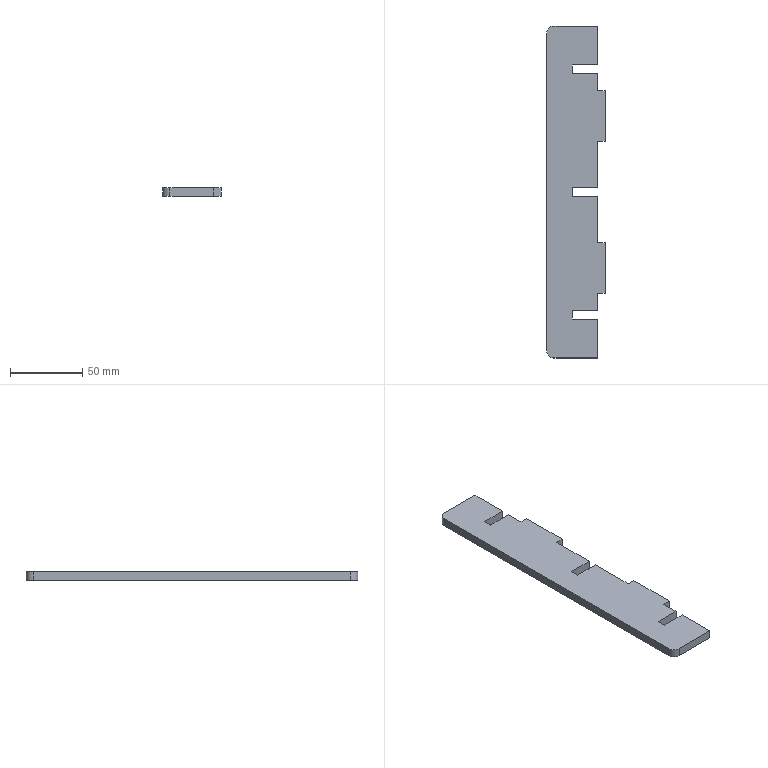Part | SolidWorks | features FlatPattern 1, SMBaseFlange 1, SheetMetal 1 | 1 solid | 28 faces | box 40.5 x 230 x 6 mm | volume 48656 mm3 | plane 26 | cylinder 2 | commonest cylinder face diameters 10 x2
STEP:
#1=CARTESIAN_POINT('',(-343.504,69.325,0.));
#2=VERTEX_POINT('',#1);
#3=CARTESIAN_POINT('',(-343.504,96.325,0.));
#4=VERTEX_POINT('',#3);
#5=CARTESIAN_POINT('',(-343.504,96.325,0.));
#6=DIRECTION('',(0.,1.,0.));
#7=VECTOR('',#6,1000.);
#8=LINE('',#5,#7);
#9=EDGE_CURVE('',#2,#4,#8,.T.);
#10=ORIENTED_EDGE('',*,*,#9,.F.);
#11=CARTESIAN_POINT('',(-343.504,69.325,-6.));
#12=VERTEX_POINT('',#11);
#13=CARTESIAN_POINT('',(-343.504,69.325,-6.));
#14=DIRECTION('',(0.,0.,1.));
#15=VECTOR('',#14,1000.);
#16=LINE('',#13,#15);
#17=EDGE_CURVE('',#12,#2,#16,.T.);
#18=ORIENTED_EDGE('',*,*,#17,.F.);
#19=CARTESIAN_POINT('',(-343.504,96.325,-6.));
#20=VERTEX_POINT('',#19);
#21=CARTESIAN_POINT('',(-343.504,96.325,-6.));
#22=DIRECTION('',(0.,1.,0.));
#23=VECTOR('',#22,1000.);
#24=LINE('',#21,#23);
#25=EDGE_CURVE('',#12,#20,#24,.T.);
#26=ORIENTED_EDGE('',*,*,#25,.T.);
#27=CARTESIAN_POINT('',(-343.504,96.325,-6.));
#28=DIRECTION('',(0.,0.,1.));
#29=VECTOR('',#28,1000.);
#30=LINE('',#27,#29);
#31=EDGE_CURVE('',#20,#4,#30,.T.);
#32=ORIENTED_EDGE('',*,*,#31,.T.);
#33=EDGE_LOOP('',(#10,#18,#26,#32));
#34=FACE_OUTER_BOUND('',#33,.T.);
#35=CARTESIAN_POINT('',(-343.504,96.325,-6.));
#36=DIRECTION('',(1.,0.,0.));
#37=DIRECTION('',(0.,1.,0.));
#38=AXIS2_PLACEMENT_3D('',#35,#36,#37);
#39=PLANE('',#38);
#40=ADVANCED_FACE('',(#34),#39,.T.);
#41=CARTESIAN_POINT('',(-361.004,69.325,0.));
#42=VERTEX_POINT('',#41);
#43=CARTESIAN_POINT('',(-343.504,69.325,0.));
#44=DIRECTION('',(1.,0.,0.));
#45=VECTOR('',#44,1000.);
#46=LINE('',#43,#45);
#47=EDGE_CURVE('',#42,#2,#46,.T.);
#48=ORIENTED_EDGE('',*,*,#47,.F.);
#49=CARTESIAN_POINT('',(-361.004,69.325,-6.));
#50=VERTEX_POINT('',#49);
#51=CARTESIAN_POINT('',(-361.004,69.325,-6.));
#52=DIRECTION('',(0.,0.,1.));
#53=VECTOR('',#52,1000.);
#54=LINE('',#51,#53);
#55=EDGE_CURVE('',#50,#42,#54,.T.);
#56=ORIENTED_EDGE('',*,*,#55,.F.);
#57=CARTESIAN_POINT('',(-343.504,69.325,-6.));
#58=DIRECTION('',(1.,0.,0.));
#59=VECTOR('',#58,1000.);
#60=LINE('',#57,#59);
#61=EDGE_CURVE('',#50,#12,#60,.T.);
#62=ORIENTED_EDGE('',*,*,#61,.T.);
#63=ORIENTED_EDGE('',*,*,#17,.T.);
#64=EDGE_LOOP('',(#48,#56,#62,#63));
#65=FACE_OUTER_BOUND('',#64,.T.);
#66=CARTESIAN_POINT('',(-343.504,69.325,-6.));
#67=DIRECTION('',(0.,-1.,0.));
#68=DIRECTION('',(0.,0.,-1.));
#69=AXIS2_PLACEMENT_3D('',#66,#67,#68);
#70=PLANE('',#69);
#71=ADVANCED_FACE('',(#65),#70,.T.);
#72=CARTESIAN_POINT('',(-361.004,63.325,0.));
#73=VERTEX_POINT('',#72);
#74=CARTESIAN_POINT('',(-361.004,69.325,0.));
#75=DIRECTION('',(0.,1.,0.));
#76=VECTOR('',#75,1000.);
#77=LINE('',#74,#76);
#78=EDGE_CURVE('',#73,#42,#77,.T.);
#79=ORIENTED_EDGE('',*,*,#78,.F.);
#80=CARTESIAN_POINT('',(-361.004,63.325,-6.));
#81=VERTEX_POINT('',#80);
#82=CARTESIAN_POINT('',(-361.004,63.325,-6.));
#83=DIRECTION('',(0.,0.,1.));
#84=VECTOR('',#83,1000.);
#85=LINE('',#82,#84);
#86=EDGE_CURVE('',#81,#73,#85,.T.);
#87=ORIENTED_EDGE('',*,*,#86,.F.);
#88=CARTESIAN_POINT('',(-361.004,69.325,-6.));
#89=DIRECTION('',(0.,1.,0.));
#90=VECTOR('',#89,1000.);
#91=LINE('',#88,#90);
#92=EDGE_CURVE('',#81,#50,#91,.T.);
#93=ORIENTED_EDGE('',*,*,#92,.T.);
#94=ORIENTED_EDGE('',*,*,#55,.T.);
#95=EDGE_LOOP('',(#79,#87,#93,#94));
#96=FACE_OUTER_BOUND('',#95,.T.);
#97=CARTESIAN_POINT('',(-361.004,69.325,-6.));
#98=DIRECTION('',(1.,0.,0.));
#99=DIRECTION('',(0.,0.,-1.));
#100=AXIS2_PLACEMENT_3D('',#97,#98,#99);
#101=PLANE('',#100);
#102=ADVANCED_FACE('',(#96),#101,.T.);
#103=CARTESIAN_POINT('',(-343.504,63.325,0.));
#104=VERTEX_POINT('',#103);
#105=CARTESIAN_POINT('',(-361.004,63.325,0.));
#106=DIRECTION('',(-1.,0.,0.));
#107=VECTOR('',#106,1000.);
#108=LINE('',#105,#107);
#109=EDGE_CURVE('',#104,#73,#108,.T.);
#110=ORIENTED_EDGE('',*,*,#109,.F.);
#111=CARTESIAN_POINT('',(-343.504,63.325,-6.));
#112=VERTEX_POINT('',#111);
#113=CARTESIAN_POINT('',(-343.504,63.325,-6.));
#114=DIRECTION('',(0.,0.,1.));
#115=VECTOR('',#114,1000.);
#116=LINE('',#113,#115);
#117=EDGE_CURVE('',#112,#104,#116,.T.);
#118=ORIENTED_EDGE('',*,*,#117,.F.);
#119=CARTESIAN_POINT('',(-361.004,63.325,-6.));
#120=DIRECTION('',(-1.,0.,0.));
#121=VECTOR('',#120,1000.);
#122=LINE('',#119,#121);
#123=EDGE_CURVE('',#112,#81,#122,.T.);
#124=ORIENTED_EDGE('',*,*,#123,.T.);
#125=ORIENTED_EDGE('',*,*,#86,.T.);
#126=EDGE_LOOP('',(#110,#118,#124,#125));
#127=FACE_OUTER_BOUND('',#126,.T.);
#128=CARTESIAN_POINT('',(-361.004,63.325,-6.));
#129=DIRECTION('',(0.,1.,0.));
#130=DIRECTION('',(0.,0.,1.));
#131=AXIS2_PLACEMENT_3D('',#128,#129,#130);
#132=PLANE('',#131);
#133=ADVANCED_FACE('',(#127),#132,.T.);
#134=CARTESIAN_POINT('',(-343.504,51.325,0.));
#135=VERTEX_POINT('',#134);
#136=CARTESIAN_POINT('',(-343.504,63.325,0.));
#137=DIRECTION('',(0.,1.,0.));
#138=VECTOR('',#137,1000.);
#139=LINE('',#136,#138);
#140=EDGE_CURVE('',#135,#104,#139,.T.);
#141=ORIENTED_EDGE('',*,*,#140,.F.);
#142=CARTESIAN_POINT('',(-343.504,51.325,-6.));
#143=VERTEX_POINT('',#142);
#144=CARTESIAN_POINT('',(-343.504,51.325,-6.));
#145=DIRECTION('',(0.,0.,1.));
#146=VECTOR('',#145,1000.);
#147=LINE('',#144,#146);
#148=EDGE_CURVE('',#143,#135,#147,.T.);
#149=ORIENTED_EDGE('',*,*,#148,.F.);
#150=CARTESIAN_POINT('',(-343.504,63.325,-6.));
#151=DIRECTION('',(0.,1.,0.));
#152=VECTOR('',#151,1000.);
#153=LINE('',#150,#152);
#154=EDGE_CURVE('',#143,#112,#153,.T.);
#155=ORIENTED_EDGE('',*,*,#154,.T.);
#156=ORIENTED_EDGE('',*,*,#117,.T.);
#157=EDGE_LOOP('',(#141,#149,#155,#156));
#158=FACE_OUTER_BOUND('',#157,.T.);
#159=CARTESIAN_POINT('',(-343.504,63.325,-6.));
#160=DIRECTION('',(1.,0.,0.));
#161=DIRECTION('',(0.,1.,0.));
#162=AXIS2_PLACEMENT_3D('',#159,#160,#161);
#163=PLANE('',#162);
#164=ADVANCED_FACE('',(#158),#163,.T.);
#165=CARTESIAN_POINT('',(-338.004,51.325,0.));
#166=VERTEX_POINT('',#165);
#167=CARTESIAN_POINT('',(-343.504,51.325,0.));
#168=DIRECTION('',(-1.,0.,0.));
#169=VECTOR('',#168,1000.);
#170=LINE('',#167,#169);
#171=EDGE_CURVE('',#166,#135,#170,.T.);
#172=ORIENTED_EDGE('',*,*,#171,.F.);
#173=CARTESIAN_POINT('',(-338.004,51.325,-6.));
#174=VERTEX_POINT('',#173);
#175=CARTESIAN_POINT('',(-338.004,51.325,-6.));
#176=DIRECTION('',(0.,0.,1.));
#177=VECTOR('',#176,1000.);
#178=LINE('',#175,#177);
#179=EDGE_CURVE('',#174,#166,#178,.T.);
#180=ORIENTED_EDGE('',*,*,#179,.F.);
#181=CARTESIAN_POINT('',(-343.504,51.325,-6.));
#182=DIRECTION('',(-1.,0.,0.));
#183=VECTOR('',#182,1000.);
#184=LINE('',#181,#183);
#185=EDGE_CURVE('',#174,#143,#184,.T.);
#186=ORIENTED_EDGE('',*,*,#185,.T.);
#187=ORIENTED_EDGE('',*,*,#148,.T.);
#188=EDGE_LOOP('',(#172,#180,#186,#187));
#189=FACE_OUTER_BOUND('',#188,.T.);
#190=CARTESIAN_POINT('',(-343.504,51.325,-6.));
#191=DIRECTION('',(0.,1.,0.));
#192=DIRECTION('',(-1.,0.,0.));
#193=AXIS2_PLACEMENT_3D('',#190,#191,#192);
#194=PLANE('',#193);
#195=ADVANCED_FACE('',(#189),#194,.T.);
#196=CARTESIAN_POINT('',(-338.004,16.325,0.));
#197=VERTEX_POINT('',#196);
#198=CARTESIAN_POINT('',(-338.004,51.325,0.));
#199=DIRECTION('',(0.,1.,0.));
#200=VECTOR('',#199,1000.);
#201=LINE('',#198,#200);
#202=EDGE_CURVE('',#197,#166,#201,.T.);
#203=ORIENTED_EDGE('',*,*,#202,.F.);
#204=CARTESIAN_POINT('',(-338.004,16.325,-6.));
#205=VERTEX_POINT('',#204);
#206=CARTESIAN_POINT('',(-338.004,16.325,-6.));
#207=DIRECTION('',(0.,0.,1.));
#208=VECTOR('',#207,1000.);
#209=LINE('',#206,#208);
#210=EDGE_CURVE('',#205,#197,#209,.T.);
#211=ORIENTED_EDGE('',*,*,#210,.F.);
#212=CARTESIAN_POINT('',(-338.004,51.325,-6.));
#213=DIRECTION('',(0.,1.,0.));
#214=VECTOR('',#213,1000.);
#215=LINE('',#212,#214);
#216=EDGE_CURVE('',#205,#174,#215,.T.);
#217=ORIENTED_EDGE('',*,*,#216,.T.);
#218=ORIENTED_EDGE('',*,*,#179,.T.);
#219=EDGE_LOOP('',(#203,#211,#217,#218));
#220=FACE_OUTER_BOUND('',#219,.T.);
#221=CARTESIAN_POINT('',(-338.004,51.325,-6.));
#222=DIRECTION('',(1.,0.,0.));
#223=DIRECTION('',(0.,0.,-1.));
#224=AXIS2_PLACEMENT_3D('',#221,#222,#223);
#225=PLANE('',#224);
#226=ADVANCED_FACE('',(#220),#225,.T.);
#227=CARTESIAN_POINT('',(-343.504,16.325,0.));
#228=VERTEX_POINT('',#227);
#229=CARTESIAN_POINT('',(-338.004,16.325,0.));
#230=DIRECTION('',(1.,0.,0.));
#231=VECTOR('',#230,1000.);
#232=LINE('',#229,#231);
#233=EDGE_CURVE('',#228,#197,#232,.T.);
#234=ORIENTED_EDGE('',*,*,#233,.F.);
#235=CARTESIAN_POINT('',(-343.504,16.325,-6.));
#236=VERTEX_POINT('',#235);
#237=CARTESIAN_POINT('',(-343.504,16.325,-6.));
#238=DIRECTION('',(0.,0.,1.));
#239=VECTOR('',#238,1000.);
#240=LINE('',#237,#239);
#241=EDGE_CURVE('',#236,#228,#240,.T.);
#242=ORIENTED_EDGE('',*,*,#241,.F.);
#243=CARTESIAN_POINT('',(-338.004,16.325,-6.));
#244=DIRECTION('',(1.,0.,0.));
#245=VECTOR('',#244,1000.);
#246=LINE('',#243,#245);
#247=EDGE_CURVE('',#236,#205,#246,.T.);
#248=ORIENTED_EDGE('',*,*,#247,.T.);
#249=ORIENTED_EDGE('',*,*,#210,.T.);
#250=EDGE_LOOP('',(#234,#242,#248,#249));
#251=FACE_OUTER_BOUND('',#250,.T.);
#252=CARTESIAN_POINT('',(-338.004,16.325,-6.));
#253=DIRECTION('',(0.,-1.,0.));
#254=DIRECTION('',(0.,0.,-1.));
#255=AXIS2_PLACEMENT_3D('',#252,#253,#254);
#256=PLANE('',#255);
#257=ADVANCED_FACE('',(#251),#256,.T.);
#258=CARTESIAN_POINT('',(-343.504,-15.675,0.));
#259=VERTEX_POINT('',#258);
#260=CARTESIAN_POINT('',(-343.504,16.325,0.));
#261=DIRECTION('',(0.,1.,0.));
#262=VECTOR('',#261,1000.);
#263=LINE('',#260,#262);
#264=EDGE_CURVE('',#259,#228,#263,.T.);
#265=ORIENTED_EDGE('',*,*,#264,.F.);
#266=CARTESIAN_POINT('',(-343.504,-15.675,-6.));
#267=VERTEX_POINT('',#266);
#268=CARTESIAN_POINT('',(-343.504,-15.675,-6.));
#269=DIRECTION('',(0.,0.,1.));
#270=VECTOR('',#269,1000.);
#271=LINE('',#268,#270);
#272=EDGE_CURVE('',#267,#259,#271,.T.);
#273=ORIENTED_EDGE('',*,*,#272,.F.);
#274=CARTESIAN_POINT('',(-343.504,16.325,-6.));
#275=DIRECTION('',(0.,1.,0.));
#276=VECTOR('',#275,1000.);
#277=LINE('',#274,#276);
#278=EDGE_CURVE('',#267,#236,#277,.T.);
#279=ORIENTED_EDGE('',*,*,#278,.T.);
#280=ORIENTED_EDGE('',*,*,#241,.T.);
#281=EDGE_LOOP('',(#265,#273,#279,#280));
#282=FACE_OUTER_BOUND('',#281,.T.);
#283=CARTESIAN_POINT('',(-343.504,16.325,-6.));
#284=DIRECTION('',(1.,0.,0.));
#285=DIRECTION('',(0.,1.,0.));
#286=AXIS2_PLACEMENT_3D('',#283,#284,#285);
#287=PLANE('',#286);
#288=ADVANCED_FACE('',(#282),#287,.T.);
#289=CARTESIAN_POINT('',(-361.004,-15.675,0.));
#290=VERTEX_POINT('',#289);
#291=CARTESIAN_POINT('',(-343.504,-15.675,0.));
#292=DIRECTION('',(1.,0.,0.));
#293=VECTOR('',#292,1000.);
#294=LINE('',#291,#293);
#295=EDGE_CURVE('',#290,#259,#294,.T.);
#296=ORIENTED_EDGE('',*,*,#295,.F.);
#297=CARTESIAN_POINT('',(-361.004,-15.675,-6.));
#298=VERTEX_POINT('',#297);
#299=CARTESIAN_POINT('',(-361.004,-15.675,-6.));
#300=DIRECTION('',(0.,0.,1.));
#301=VECTOR('',#300,1000.);
#302=LINE('',#299,#301);
#303=EDGE_CURVE('',#298,#290,#302,.T.);
#304=ORIENTED_EDGE('',*,*,#303,.F.);
#305=CARTESIAN_POINT('',(-343.504,-15.675,-6.));
#306=DIRECTION('',(1.,0.,0.));
#307=VECTOR('',#306,1000.);
#308=LINE('',#305,#307);
#309=EDGE_CURVE('',#298,#267,#308,.T.);
#310=ORIENTED_EDGE('',*,*,#309,.T.);
#311=ORIENTED_EDGE('',*,*,#272,.T.);
#312=EDGE_LOOP('',(#296,#304,#310,#311));
#313=FACE_OUTER_BOUND('',#312,.T.);
#314=CARTESIAN_POINT('',(-343.504,-15.675,-6.));
#315=DIRECTION('',(0.,-1.,0.));
#316=DIRECTION('',(0.,0.,-1.));
#317=AXIS2_PLACEMENT_3D('',#314,#315,#316);
#318=PLANE('',#317);
#319=ADVANCED_FACE('',(#313),#318,.T.);
#320=CARTESIAN_POINT('',(-361.004,-21.675,0.));
#321=VERTEX_POINT('',#320);
#322=CARTESIAN_POINT('',(-361.004,-15.675,0.));
#323=DIRECTION('',(0.,1.,0.));
#324=VECTOR('',#323,1000.);
#325=LINE('',#322,#324);
#326=EDGE_CURVE('',#321,#290,#325,.T.);
#327=ORIENTED_EDGE('',*,*,#326,.F.);
#328=CARTESIAN_POINT('',(-361.004,-21.675,-6.));
#329=VERTEX_POINT('',#328);
#330=CARTESIAN_POINT('',(-361.004,-21.675,-6.));
#331=DIRECTION('',(0.,0.,1.));
#332=VECTOR('',#331,1000.);
#333=LINE('',#330,#332);
#334=EDGE_CURVE('',#329,#321,#333,.T.);
#335=ORIENTED_EDGE('',*,*,#334,.F.);
#336=CARTESIAN_POINT('',(-361.004,-15.675,-6.));
#337=DIRECTION('',(0.,1.,0.));
#338=VECTOR('',#337,1000.);
#339=LINE('',#336,#338);
#340=EDGE_CURVE('',#329,#298,#339,.T.);
#341=ORIENTED_EDGE('',*,*,#340,.T.);
#342=ORIENTED_EDGE('',*,*,#303,.T.);
#343=EDGE_LOOP('',(#327,#335,#341,#342));
#344=FACE_OUTER_BOUND('',#343,.T.);
#345=CARTESIAN_POINT('',(-361.004,-15.675,-6.));
#346=DIRECTION('',(1.,0.,0.));
#347=DIRECTION('',(0.,0.,-1.));
#348=AXIS2_PLACEMENT_3D('',#345,#346,#347);
#349=PLANE('',#348);
#350=ADVANCED_FACE('',(#344),#349,.T.);
#351=CARTESIAN_POINT('',(-343.504,-21.675,0.));
#352=VERTEX_POINT('',#351);
#353=CARTESIAN_POINT('',(-361.004,-21.675,0.));
#354=DIRECTION('',(-1.,0.,0.));
#355=VECTOR('',#354,1000.);
#356=LINE('',#353,#355);
#357=EDGE_CURVE('',#352,#321,#356,.T.);
#358=ORIENTED_EDGE('',*,*,#357,.F.);
#359=CARTESIAN_POINT('',(-343.504,-21.675,-6.));
#360=VERTEX_POINT('',#359);
#361=CARTESIAN_POINT('',(-343.504,-21.675,-6.));
#362=DIRECTION('',(0.,0.,1.));
#363=VECTOR('',#362,1000.);
#364=LINE('',#361,#363);
#365=EDGE_CURVE('',#360,#352,#364,.T.);
#366=ORIENTED_EDGE('',*,*,#365,.F.);
#367=CARTESIAN_POINT('',(-361.004,-21.675,-6.));
#368=DIRECTION('',(-1.,0.,0.));
#369=VECTOR('',#368,1000.);
#370=LINE('',#367,#369);
#371=EDGE_CURVE('',#360,#329,#370,.T.);
#372=ORIENTED_EDGE('',*,*,#371,.T.);
#373=ORIENTED_EDGE('',*,*,#334,.T.);
#374=EDGE_LOOP('',(#358,#366,#372,#373));
#375=FACE_OUTER_BOUND('',#374,.T.);
#376=CARTESIAN_POINT('',(-361.004,-21.675,-6.));
#377=DIRECTION('',(0.,1.,0.));
#378=DIRECTION('',(0.,0.,1.));
#379=AXIS2_PLACEMENT_3D('',#376,#377,#378);
#380=PLANE('',#379);
#381=ADVANCED_FACE('',(#375),#380,.T.);
#382=CARTESIAN_POINT('',(-343.504,-53.675,0.));
#383=VERTEX_POINT('',#382);
#384=CARTESIAN_POINT('',(-343.504,-21.675,0.));
#385=DIRECTION('',(0.,1.,0.));
#386=VECTOR('',#385,1000.);
#387=LINE('',#384,#386);
#388=EDGE_CURVE('',#383,#352,#387,.T.);
#389=ORIENTED_EDGE('',*,*,#388,.F.);
#390=CARTESIAN_POINT('',(-343.504,-53.675,-6.));
#391=VERTEX_POINT('',#390);
#392=CARTESIAN_POINT('',(-343.504,-53.675,-6.));
#393=DIRECTION('',(0.,0.,1.));
#394=VECTOR('',#393,1000.);
#395=LINE('',#392,#394);
#396=EDGE_CURVE('',#391,#383,#395,.T.);
#397=ORIENTED_EDGE('',*,*,#396,.F.);
#398=CARTESIAN_POINT('',(-343.504,-21.675,-6.));
#399=DIRECTION('',(0.,1.,0.));
#400=VECTOR('',#399,1000.);
#401=LINE('',#398,#400);
#402=EDGE_CURVE('',#391,#360,#401,.T.);
#403=ORIENTED_EDGE('',*,*,#402,.T.);
#404=ORIENTED_EDGE('',*,*,#365,.T.);
#405=EDGE_LOOP('',(#389,#397,#403,#404));
#406=FACE_OUTER_BOUND('',#405,.T.);
#407=CARTESIAN_POINT('',(-343.504,-21.675,-6.));
#408=DIRECTION('',(1.,0.,0.));
#409=DIRECTION('',(0.,1.,0.));
#410=AXIS2_PLACEMENT_3D('',#407,#408,#409);
#411=PLANE('',#410);
#412=ADVANCED_FACE('',(#406),#411,.T.);
#413=CARTESIAN_POINT('',(-338.004,-53.675,0.));
#414=VERTEX_POINT('',#413);
#415=CARTESIAN_POINT('',(-343.504,-53.675,0.));
#416=DIRECTION('',(-1.,0.,0.));
#417=VECTOR('',#416,1000.);
#418=LINE('',#415,#417);
#419=EDGE_CURVE('',#414,#383,#418,.T.);
#420=ORIENTED_EDGE('',*,*,#419,.F.);
#421=CARTESIAN_POINT('',(-338.004,-53.675,-6.));
#422=VERTEX_POINT('',#421);
#423=CARTESIAN_POINT('',(-338.004,-53.675,-6.));
#424=DIRECTION('',(0.,0.,1.));
#425=VECTOR('',#424,1000.);
#426=LINE('',#423,#425);
#427=EDGE_CURVE('',#422,#414,#426,.T.);
#428=ORIENTED_EDGE('',*,*,#427,.F.);
#429=CARTESIAN_POINT('',(-343.504,-53.675,-6.));
#430=DIRECTION('',(-1.,0.,0.));
#431=VECTOR('',#430,1000.);
#432=LINE('',#429,#431);
#433=EDGE_CURVE('',#422,#391,#432,.T.);
#434=ORIENTED_EDGE('',*,*,#433,.T.);
#435=ORIENTED_EDGE('',*,*,#396,.T.);
#436=EDGE_LOOP('',(#420,#428,#434,#435));
#437=FACE_OUTER_BOUND('',#436,.T.);
#438=CARTESIAN_POINT('',(-343.504,-53.675,-6.));
#439=DIRECTION('',(0.,1.,0.));
#440=DIRECTION('',(0.,0.,1.));
#441=AXIS2_PLACEMENT_3D('',#438,#439,#440);
#442=PLANE('',#441);
#443=ADVANCED_FACE('',(#437),#442,.T.);
#444=CARTESIAN_POINT('',(-338.004,-88.675,0.));
#445=VERTEX_POINT('',#444);
#446=CARTESIAN_POINT('',(-338.004,-53.675,0.));
#447=DIRECTION('',(0.,1.,0.));
#448=VECTOR('',#447,1000.);
#449=LINE('',#446,#448);
#450=EDGE_CURVE('',#445,#414,#449,.T.);
#451=ORIENTED_EDGE('',*,*,#450,.F.);
#452=CARTESIAN_POINT('',(-338.004,-88.675,-6.));
#453=VERTEX_POINT('',#452);
#454=CARTESIAN_POINT('',(-338.004,-88.675,-6.));
#455=DIRECTION('',(0.,0.,1.));
#456=VECTOR('',#455,1000.);
#457=LINE('',#454,#456);
#458=EDGE_CURVE('',#453,#445,#457,.T.);
#459=ORIENTED_EDGE('',*,*,#458,.F.);
#460=CARTESIAN_POINT('',(-338.004,-53.675,-6.));
#461=DIRECTION('',(0.,1.,0.));
#462=VECTOR('',#461,1000.);
#463=LINE('',#460,#462);
#464=EDGE_CURVE('',#453,#422,#463,.T.);
#465=ORIENTED_EDGE('',*,*,#464,.T.);
#466=ORIENTED_EDGE('',*,*,#427,.T.);
#467=EDGE_LOOP('',(#451,#459,#465,#466));
#468=FACE_OUTER_BOUND('',#467,.T.);
#469=CARTESIAN_POINT('',(-338.004,-53.675,-6.));
#470=DIRECTION('',(1.,0.,0.));
#471=DIRECTION('',(0.,0.,-1.));
#472=AXIS2_PLACEMENT_3D('',#469,#470,#471);
#473=PLANE('',#472);
#474=ADVANCED_FACE('',(#468),#473,.T.);
#475=CARTESIAN_POINT('',(-343.504,-88.675,0.));
#476=VERTEX_POINT('',#475);
#477=CARTESIAN_POINT('',(-338.004,-88.675,0.));
#478=DIRECTION('',(1.,0.,0.));
#479=VECTOR('',#478,1000.);
#480=LINE('',#477,#479);
#481=EDGE_CURVE('',#476,#445,#480,.T.);
#482=ORIENTED_EDGE('',*,*,#481,.F.);
#483=CARTESIAN_POINT('',(-343.504,-88.675,-6.));
#484=VERTEX_POINT('',#483);
#485=CARTESIAN_POINT('',(-343.504,-88.675,-6.));
#486=DIRECTION('',(0.,0.,1.));
#487=VECTOR('',#486,1000.);
#488=LINE('',#485,#487);
#489=EDGE_CURVE('',#484,#476,#488,.T.);
#490=ORIENTED_EDGE('',*,*,#489,.F.);
#491=CARTESIAN_POINT('',(-338.004,-88.675,-6.));
#492=DIRECTION('',(1.,0.,0.));
#493=VECTOR('',#492,1000.);
#494=LINE('',#491,#493);
#495=EDGE_CURVE('',#484,#453,#494,.T.);
#496=ORIENTED_EDGE('',*,*,#495,.T.);
#497=ORIENTED_EDGE('',*,*,#458,.T.);
#498=EDGE_LOOP('',(#482,#490,#496,#497));
#499=FACE_OUTER_BOUND('',#498,.T.);
#500=CARTESIAN_POINT('',(-338.004,-88.675,-6.));
#501=DIRECTION('',(0.,-1.,0.));
#502=DIRECTION('',(0.,0.,-1.));
#503=AXIS2_PLACEMENT_3D('',#500,#501,#502);
#504=PLANE('',#503);
#505=ADVANCED_FACE('',(#499),#504,.T.);
#506=CARTESIAN_POINT('',(-343.504,-100.675,0.));
#507=VERTEX_POINT('',#506);
#508=CARTESIAN_POINT('',(-343.504,-88.675,0.));
#509=DIRECTION('',(0.,1.,0.));
#510=VECTOR('',#509,1000.);
#511=LINE('',#508,#510);
#512=EDGE_CURVE('',#507,#476,#511,.T.);
#513=ORIENTED_EDGE('',*,*,#512,.F.);
#514=CARTESIAN_POINT('',(-343.504,-100.675,-6.));
#515=VERTEX_POINT('',#514);
#516=CARTESIAN_POINT('',(-343.504,-100.675,-6.));
#517=DIRECTION('',(0.,0.,1.));
#518=VECTOR('',#517,1000.);
#519=LINE('',#516,#518);
#520=EDGE_CURVE('',#515,#507,#519,.T.);
#521=ORIENTED_EDGE('',*,*,#520,.F.);
#522=CARTESIAN_POINT('',(-343.504,-88.675,-6.));
#523=DIRECTION('',(0.,1.,0.));
#524=VECTOR('',#523,1000.);
#525=LINE('',#522,#524);
#526=EDGE_CURVE('',#515,#484,#525,.T.);
#527=ORIENTED_EDGE('',*,*,#526,.T.);
#528=ORIENTED_EDGE('',*,*,#489,.T.);
#529=EDGE_LOOP('',(#513,#521,#527,#528));
#530=FACE_OUTER_BOUND('',#529,.T.);
#531=CARTESIAN_POINT('',(-343.504,-88.675,-6.));
#532=DIRECTION('',(1.,0.,0.));
#533=DIRECTION('',(0.,0.,-1.));
#534=AXIS2_PLACEMENT_3D('',#531,#532,#533);
#535=PLANE('',#534);
#536=ADVANCED_FACE('',(#530),#535,.T.);
#537=CARTESIAN_POINT('',(-361.004,-100.675,0.));
#538=VERTEX_POINT('',#537);
#539=CARTESIAN_POINT('',(-343.504,-100.675,0.));
#540=DIRECTION('',(1.,0.,0.));
#541=VECTOR('',#540,1000.);
#542=LINE('',#539,#541);
#543=EDGE_CURVE('',#538,#507,#542,.T.);
#544=ORIENTED_EDGE('',*,*,#543,.F.);
#545=CARTESIAN_POINT('',(-361.004,-100.675,-6.));
#546=VERTEX_POINT('',#545);
#547=CARTESIAN_POINT('',(-361.004,-100.675,-6.));
#548=DIRECTION('',(0.,0.,1.));
#549=VECTOR('',#548,1000.);
#550=LINE('',#547,#549);
#551=EDGE_CURVE('',#546,#538,#550,.T.);
#552=ORIENTED_EDGE('',*,*,#551,.F.);
#553=CARTESIAN_POINT('',(-343.504,-100.675,-6.));
#554=DIRECTION('',(1.,0.,0.));
#555=VECTOR('',#554,1000.);
#556=LINE('',#553,#555);
#557=EDGE_CURVE('',#546,#515,#556,.T.);
#558=ORIENTED_EDGE('',*,*,#557,.T.);
#559=ORIENTED_EDGE('',*,*,#520,.T.);
#560=EDGE_LOOP('',(#544,#552,#558,#559));
#561=FACE_OUTER_BOUND('',#560,.T.);
#562=CARTESIAN_POINT('',(-343.504,-100.675,-6.));
#563=DIRECTION('',(0.,-1.,0.));
#564=DIRECTION('',(0.,0.,-1.));
#565=AXIS2_PLACEMENT_3D('',#562,#563,#564);
#566=PLANE('',#565);
#567=ADVANCED_FACE('',(#561),#566,.T.);
#568=CARTESIAN_POINT('',(-361.004,-106.675,0.));
#569=VERTEX_POINT('',#568);
#570=CARTESIAN_POINT('',(-361.004,-100.675,0.));
#571=DIRECTION('',(0.,1.,0.));
#572=VECTOR('',#571,1000.);
#573=LINE('',#570,#572);
#574=EDGE_CURVE('',#569,#538,#573,.T.);
#575=ORIENTED_EDGE('',*,*,#574,.F.);
#576=CARTESIAN_POINT('',(-361.004,-106.675,-6.));
#577=VERTEX_POINT('',#576);
#578=CARTESIAN_POINT('',(-361.004,-106.675,-6.));
#579=DIRECTION('',(0.,0.,1.));
#580=VECTOR('',#579,1000.);
#581=LINE('',#578,#580);
#582=EDGE_CURVE('',#577,#569,#581,.T.);
#583=ORIENTED_EDGE('',*,*,#582,.F.);
#584=CARTESIAN_POINT('',(-361.004,-100.675,-6.));
#585=DIRECTION('',(0.,1.,0.));
#586=VECTOR('',#585,1000.);
#587=LINE('',#584,#586);
#588=EDGE_CURVE('',#577,#546,#587,.T.);
#589=ORIENTED_EDGE('',*,*,#588,.T.);
#590=ORIENTED_EDGE('',*,*,#551,.T.);
#591=EDGE_LOOP('',(#575,#583,#589,#590));
#592=FACE_OUTER_BOUND('',#591,.T.);
#593=CARTESIAN_POINT('',(-361.004,-100.675,-6.));
#594=DIRECTION('',(1.,0.,0.));
#595=DIRECTION('',(0.,0.,-1.));
#596=AXIS2_PLACEMENT_3D('',#593,#594,#595);
#597=PLANE('',#596);
#598=ADVANCED_FACE('',(#592),#597,.T.);
#599=CARTESIAN_POINT('',(-343.504,-106.675,0.));
#600=VERTEX_POINT('',#599);
#601=CARTESIAN_POINT('',(-361.004,-106.675,0.));
#602=DIRECTION('',(-1.,0.,0.));
#603=VECTOR('',#602,1000.);
#604=LINE('',#601,#603);
#605=EDGE_CURVE('',#600,#569,#604,.T.);
#606=ORIENTED_EDGE('',*,*,#605,.F.);
#607=CARTESIAN_POINT('',(-343.504,-106.675,-6.));
#608=VERTEX_POINT('',#607);
#609=CARTESIAN_POINT('',(-343.504,-106.675,-6.));
#610=DIRECTION('',(0.,0.,1.));
#611=VECTOR('',#610,1000.);
#612=LINE('',#609,#611);
#613=EDGE_CURVE('',#608,#600,#612,.T.);
#614=ORIENTED_EDGE('',*,*,#613,.F.);
#615=CARTESIAN_POINT('',(-361.004,-106.675,-6.));
#616=DIRECTION('',(-1.,0.,0.));
#617=VECTOR('',#616,1000.);
#618=LINE('',#615,#617);
#619=EDGE_CURVE('',#608,#577,#618,.T.);
#620=ORIENTED_EDGE('',*,*,#619,.T.);
#621=ORIENTED_EDGE('',*,*,#582,.T.);
#622=EDGE_LOOP('',(#606,#614,#620,#621));
#623=FACE_OUTER_BOUND('',#622,.T.);
#624=CARTESIAN_POINT('',(-361.004,-106.675,-6.));
#625=DIRECTION('',(0.,1.,0.));
#626=DIRECTION('',(0.,0.,1.));
#627=AXIS2_PLACEMENT_3D('',#624,#625,#626);
#628=PLANE('',#627);
#629=ADVANCED_FACE('',(#623),#628,.T.);
#630=CARTESIAN_POINT('',(-343.504,-133.675,0.));
#631=VERTEX_POINT('',#630);
#632=CARTESIAN_POINT('',(-343.504,-106.675,0.));
#633=DIRECTION('',(0.,1.,0.));
#634=VECTOR('',#633,1000.);
#635=LINE('',#632,#634);
#636=EDGE_CURVE('',#631,#600,#635,.T.);
#637=ORIENTED_EDGE('',*,*,#636,.F.);
#638=CARTESIAN_POINT('',(-343.504,-133.675,-6.));
#639=VERTEX_POINT('',#638);
#640=CARTESIAN_POINT('',(-343.504,-133.675,-6.));
#641=DIRECTION('',(0.,0.,1.));
#642=VECTOR('',#641,1000.);
#643=LINE('',#640,#642);
#644=EDGE_CURVE('',#639,#631,#643,.T.);
#645=ORIENTED_EDGE('',*,*,#644,.F.);
#646=CARTESIAN_POINT('',(-343.504,-106.675,-6.));
#647=DIRECTION('',(0.,1.,0.));
#648=VECTOR('',#647,1000.);
#649=LINE('',#646,#648);
#650=EDGE_CURVE('',#639,#608,#649,.T.);
#651=ORIENTED_EDGE('',*,*,#650,.T.);
#652=ORIENTED_EDGE('',*,*,#613,.T.);
#653=EDGE_LOOP('',(#637,#645,#651,#652));
#654=FACE_OUTER_BOUND('',#653,.T.);
#655=CARTESIAN_POINT('',(-343.504,-106.675,-6.));
#656=DIRECTION('',(1.,0.,0.));
#657=DIRECTION('',(0.,0.,-1.));
#658=AXIS2_PLACEMENT_3D('',#655,#656,#657);
#659=PLANE('',#658);
#660=ADVANCED_FACE('',(#654),#659,.T.);
#661=CARTESIAN_POINT('',(-373.504,-133.675,0.));
#662=VERTEX_POINT('',#661);
#663=CARTESIAN_POINT('',(-343.504,-133.675,0.));
#664=DIRECTION('',(1.,0.,0.));
#665=VECTOR('',#664,1000.);
#666=LINE('',#663,#665);
#667=EDGE_CURVE('',#662,#631,#666,.T.);
#668=ORIENTED_EDGE('',*,*,#667,.F.);
#669=CARTESIAN_POINT('',(-373.504,-133.675,-6.));
#670=VERTEX_POINT('',#669);
#671=CARTESIAN_POINT('',(-373.504,-133.675,-6.));
#672=DIRECTION('',(0.,0.,1.));
#673=VECTOR('',#672,1000.);
#674=LINE('',#671,#673);
#675=EDGE_CURVE('',#670,#662,#674,.T.);
#676=ORIENTED_EDGE('',*,*,#675,.F.);
#677=CARTESIAN_POINT('',(-343.504,-133.675,-6.));
#678=DIRECTION('',(1.,0.,0.));
#679=VECTOR('',#678,1000.);
#680=LINE('',#677,#679);
#681=EDGE_CURVE('',#670,#639,#680,.T.);
#682=ORIENTED_EDGE('',*,*,#681,.T.);
#683=ORIENTED_EDGE('',*,*,#644,.T.);
#684=EDGE_LOOP('',(#668,#676,#682,#683));
#685=FACE_OUTER_BOUND('',#684,.T.);
#686=CARTESIAN_POINT('',(-343.504,-133.675,-6.));
#687=DIRECTION('',(0.,-1.,0.));
#688=DIRECTION('',(0.,0.,-1.));
#689=AXIS2_PLACEMENT_3D('',#686,#687,#688);
#690=PLANE('',#689);
#691=ADVANCED_FACE('',(#685),#690,.T.);
#692=CARTESIAN_POINT('',(-378.504,-128.675,0.));
#693=VERTEX_POINT('',#692);
#694=CARTESIAN_POINT('',(-373.504,-128.675,0.));
#695=DIRECTION('',(0.,0.,1.));
#696=DIRECTION('',(-1.,0.,0.));
#697=AXIS2_PLACEMENT_3D('',#694,#695,#696);
#698=CIRCLE('',#697,5.);
#699=EDGE_CURVE('',#693,#662,#698,.T.);
#700=ORIENTED_EDGE('',*,*,#699,.F.);
#701=CARTESIAN_POINT('',(-378.504,-128.675,-6.));
#702=VERTEX_POINT('',#701);
#703=CARTESIAN_POINT('',(-378.504,-128.675,-6.));
#704=DIRECTION('',(0.,0.,1.));
#705=VECTOR('',#704,1000.);
#706=LINE('',#703,#705);
#707=EDGE_CURVE('',#702,#693,#706,.T.);
#708=ORIENTED_EDGE('',*,*,#707,.F.);
#709=CARTESIAN_POINT('',(-373.504,-128.675,-6.));
#710=DIRECTION('',(0.,0.,1.));
#711=DIRECTION('',(-1.,0.,0.));
#712=AXIS2_PLACEMENT_3D('',#709,#710,#711);
#713=CIRCLE('',#712,5.);
#714=EDGE_CURVE('',#702,#670,#713,.T.);
#715=ORIENTED_EDGE('',*,*,#714,.T.);
#716=ORIENTED_EDGE('',*,*,#675,.T.);
#717=EDGE_LOOP('',(#700,#708,#715,#716));
#718=FACE_OUTER_BOUND('',#717,.T.);
#719=CARTESIAN_POINT('',(-373.504,-128.675,-6.));
#720=DIRECTION('',(0.,0.,1.));
#721=DIRECTION('',(1.,0.,0.));
#722=AXIS2_PLACEMENT_3D('',#719,#720,#721);
#723=CYLINDRICAL_SURFACE('',#722,5.);
#724=ADVANCED_FACE('',(#718),#723,.T.);
#725=CARTESIAN_POINT('',(-378.504,91.325,0.));
#726=VERTEX_POINT('',#725);
#727=CARTESIAN_POINT('',(-378.504,91.325,0.));
#728=DIRECTION('',(0.,-1.,0.));
#729=VECTOR('',#728,1000.);
#730=LINE('',#727,#729);
#731=EDGE_CURVE('',#726,#693,#730,.T.);
#732=ORIENTED_EDGE('',*,*,#731,.F.);
#733=CARTESIAN_POINT('',(-378.504,91.325,-6.));
#734=VERTEX_POINT('',#733);
#735=CARTESIAN_POINT('',(-378.504,91.325,-6.));
#736=DIRECTION('',(0.,0.,1.));
#737=VECTOR('',#736,1000.);
#738=LINE('',#735,#737);
#739=EDGE_CURVE('',#734,#726,#738,.T.);
#740=ORIENTED_EDGE('',*,*,#739,.F.);
#741=CARTESIAN_POINT('',(-378.504,91.325,-6.));
#742=DIRECTION('',(0.,-1.,0.));
#743=VECTOR('',#742,1000.);
#744=LINE('',#741,#743);
#745=EDGE_CURVE('',#734,#702,#744,.T.);
#746=ORIENTED_EDGE('',*,*,#745,.T.);
#747=ORIENTED_EDGE('',*,*,#707,.T.);
#748=EDGE_LOOP('',(#732,#740,#746,#747));
#749=FACE_OUTER_BOUND('',#748,.T.);
#750=CARTESIAN_POINT('',(-378.504,91.325,-6.));
#751=DIRECTION('',(-1.,0.,0.));
#752=DIRECTION('',(0.,0.,1.));
#753=AXIS2_PLACEMENT_3D('',#750,#751,#752);
#754=PLANE('',#753);
#755=ADVANCED_FACE('',(#749),#754,.T.);
#756=CARTESIAN_POINT('',(-373.504,96.325,0.));
#757=VERTEX_POINT('',#756);
#758=CARTESIAN_POINT('',(-373.504,91.325,0.));
#759=DIRECTION('',(0.,0.,1.));
#760=DIRECTION('',(1.,0.,0.));
#761=AXIS2_PLACEMENT_3D('',#758,#759,#760);
#762=CIRCLE('',#761,5.);
#763=EDGE_CURVE('',#757,#726,#762,.T.);
#764=ORIENTED_EDGE('',*,*,#763,.F.);
#765=CARTESIAN_POINT('',(-373.504,96.325,-6.));
#766=VERTEX_POINT('',#765);
#767=CARTESIAN_POINT('',(-373.504,96.325,-6.));
#768=DIRECTION('',(0.,0.,1.));
#769=VECTOR('',#768,1000.);
#770=LINE('',#767,#769);
#771=EDGE_CURVE('',#766,#757,#770,.T.);
#772=ORIENTED_EDGE('',*,*,#771,.F.);
#773=CARTESIAN_POINT('',(-373.504,91.325,-6.));
#774=DIRECTION('',(0.,0.,1.));
#775=DIRECTION('',(1.,0.,0.));
#776=AXIS2_PLACEMENT_3D('',#773,#774,#775);
#777=CIRCLE('',#776,5.);
#778=EDGE_CURVE('',#766,#734,#777,.T.);
#779=ORIENTED_EDGE('',*,*,#778,.T.);
#780=ORIENTED_EDGE('',*,*,#739,.T.);
#781=EDGE_LOOP('',(#764,#772,#779,#780));
#782=FACE_OUTER_BOUND('',#781,.T.);
#783=CARTESIAN_POINT('',(-373.504,91.325,-6.));
#784=DIRECTION('',(0.,0.,1.));
#785=DIRECTION('',(1.,0.,0.));
#786=AXIS2_PLACEMENT_3D('',#783,#784,#785);
#787=CYLINDRICAL_SURFACE('',#786,5.);
#788=ADVANCED_FACE('',(#782),#787,.T.);
#789=CARTESIAN_POINT('',(-343.504,96.325,0.));
#790=DIRECTION('',(-1.,0.,0.));
#791=VECTOR('',#790,1000.);
#792=LINE('',#789,#791);
#793=EDGE_CURVE('',#4,#757,#792,.T.);
#794=ORIENTED_EDGE('',*,*,#793,.F.);
#795=ORIENTED_EDGE('',*,*,#31,.F.);
#796=CARTESIAN_POINT('',(-343.504,96.325,-6.));
#797=DIRECTION('',(-1.,0.,0.));
#798=VECTOR('',#797,1000.);
#799=LINE('',#796,#798);
#800=EDGE_CURVE('',#20,#766,#799,.T.);
#801=ORIENTED_EDGE('',*,*,#800,.T.);
#802=ORIENTED_EDGE('',*,*,#771,.T.);
#803=EDGE_LOOP('',(#794,#795,#801,#802));
#804=FACE_OUTER_BOUND('',#803,.T.);
#805=CARTESIAN_POINT('',(-343.504,96.325,-6.));
#806=DIRECTION('',(0.,1.,0.));
#807=DIRECTION('',(0.,0.,1.));
#808=AXIS2_PLACEMENT_3D('',#805,#806,#807);
#809=PLANE('',#808);
#810=ADVANCED_FACE('',(#804),#809,.T.);
#811=ORIENTED_EDGE('',*,*,#25,.F.);
#812=ORIENTED_EDGE('',*,*,#61,.F.);
#813=ORIENTED_EDGE('',*,*,#92,.F.);
#814=ORIENTED_EDGE('',*,*,#123,.F.);
#815=ORIENTED_EDGE('',*,*,#154,.F.);
#816=ORIENTED_EDGE('',*,*,#185,.F.);
#817=ORIENTED_EDGE('',*,*,#216,.F.);
#818=ORIENTED_EDGE('',*,*,#247,.F.);
#819=ORIENTED_EDGE('',*,*,#278,.F.);
#820=ORIENTED_EDGE('',*,*,#309,.F.);
#821=ORIENTED_EDGE('',*,*,#340,.F.);
#822=ORIENTED_EDGE('',*,*,#371,.F.);
#823=ORIENTED_EDGE('',*,*,#402,.F.);
#824=ORIENTED_EDGE('',*,*,#433,.F.);
#825=ORIENTED_EDGE('',*,*,#464,.F.);
#826=ORIENTED_EDGE('',*,*,#495,.F.);
#827=ORIENTED_EDGE('',*,*,#526,.F.);
#828=ORIENTED_EDGE('',*,*,#557,.F.);
#829=ORIENTED_EDGE('',*,*,#588,.F.);
#830=ORIENTED_EDGE('',*,*,#619,.F.);
#831=ORIENTED_EDGE('',*,*,#650,.F.);
#832=ORIENTED_EDGE('',*,*,#681,.F.);
#833=ORIENTED_EDGE('',*,*,#714,.F.);
#834=ORIENTED_EDGE('',*,*,#745,.F.);
#835=ORIENTED_EDGE('',*,*,#778,.F.);
#836=ORIENTED_EDGE('',*,*,#800,.F.);
#837=EDGE_LOOP('',(#811,#812,#813,#814,#815,#816,#817,#818,#819,#820,#821,#822,#823,#824,#825,#826,#827,#828,#829,#830,#831,#832,#833,#834,#835,#836));
#838=FACE_OUTER_BOUND('',#837,.T.);
#839=CARTESIAN_POINT('',(-373.504,-128.675,-6.));
#840=DIRECTION('',(0.,0.,-1.));
#841=DIRECTION('',(-1.,0.,0.));
#842=AXIS2_PLACEMENT_3D('',#839,#840,#841);
#843=PLANE('',#842);
#844=ADVANCED_FACE('',(#838),#843,.T.);
#845=ORIENTED_EDGE('',*,*,#9,.T.);
#846=ORIENTED_EDGE('',*,*,#793,.T.);
#847=ORIENTED_EDGE('',*,*,#763,.T.);
#848=ORIENTED_EDGE('',*,*,#731,.T.);
#849=ORIENTED_EDGE('',*,*,#699,.T.);
#850=ORIENTED_EDGE('',*,*,#667,.T.);
#851=ORIENTED_EDGE('',*,*,#636,.T.);
#852=ORIENTED_EDGE('',*,*,#605,.T.);
#853=ORIENTED_EDGE('',*,*,#574,.T.);
#854=ORIENTED_EDGE('',*,*,#543,.T.);
#855=ORIENTED_EDGE('',*,*,#512,.T.);
#856=ORIENTED_EDGE('',*,*,#481,.T.);
#857=ORIENTED_EDGE('',*,*,#450,.T.);
#858=ORIENTED_EDGE('',*,*,#419,.T.);
#859=ORIENTED_EDGE('',*,*,#388,.T.);
#860=ORIENTED_EDGE('',*,*,#357,.T.);
#861=ORIENTED_EDGE('',*,*,#326,.T.);
#862=ORIENTED_EDGE('',*,*,#295,.T.);
#863=ORIENTED_EDGE('',*,*,#264,.T.);
#864=ORIENTED_EDGE('',*,*,#233,.T.);
#865=ORIENTED_EDGE('',*,*,#202,.T.);
#866=ORIENTED_EDGE('',*,*,#171,.T.);
#867=ORIENTED_EDGE('',*,*,#140,.T.);
#868=ORIENTED_EDGE('',*,*,#109,.T.);
#869=ORIENTED_EDGE('',*,*,#78,.T.);
#870=ORIENTED_EDGE('',*,*,#47,.T.);
#871=EDGE_LOOP('',(#845,#846,#847,#848,#849,#850,#851,#852,#853,#854,#855,#856,#857,#858,#859,#860,#861,#862,#863,#864,#865,#866,#867,#868,#869,#870));
#872=FACE_OUTER_BOUND('',#871,.T.);
#873=CARTESIAN_POINT('',(-373.504,-128.675,0.));
#874=DIRECTION('',(0.,0.,-1.));
#875=DIRECTION('',(-1.,0.,0.));
#876=AXIS2_PLACEMENT_3D('',#873,#874,#875);
#877=PLANE('',#876);
#878=ADVANCED_FACE('',(#872),#877,.F.);
#879=CLOSED_SHELL('',(#40,#71,#102,#133,#164,#195,#226,#257,#288,#319,#350,#381,#412,#443,#474,#505,#536,#567,#598,#629,#660,#691,#724,#755,#788,#810,#844,#878));
#880=MANIFOLD_SOLID_BREP('',#879);
#881=CARTESIAN_POINT('',(0.,0.,0.));
#882=DIRECTION('',(0.,0.,1.));
#883=DIRECTION('',(1.,0.,0.));
#884=AXIS2_PLACEMENT_3D('',#881,#882,#883);
#885=(LENGTH_UNIT()NAMED_UNIT(*)SI_UNIT(.MILLI.,.METRE.));
#886=UNCERTAINTY_MEASURE_WITH_UNIT(LENGTH_MEASURE(0.00001),#885,'','');
#887=(NAMED_UNIT(*)PLANE_ANGLE_UNIT()SI_UNIT($,.RADIAN.));
#888=(NAMED_UNIT(*)SI_UNIT($,.STERADIAN.)SOLID_ANGLE_UNIT());
#889=(GEOMETRIC_REPRESENTATION_CONTEXT(3)GLOBAL_UNCERTAINTY_ASSIGNED_CONTEXT((#886))GLOBAL_UNIT_ASSIGNED_CONTEXT((#885,#887,#888))REPRESENTATION_CONTEXT('',''));
#890=ADVANCED_BREP_SHAPE_REPRESENTATION('',(#880,#884),#889);